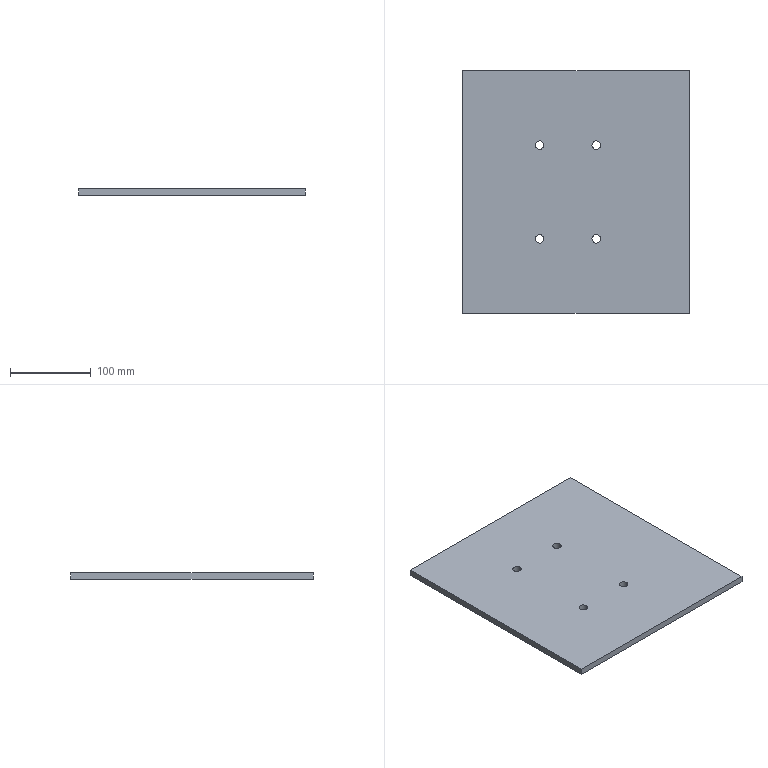Part | SolidWorks | features Extrusion 1, ICE 1 | 1 solid | 14 faces | box 280 x 300 x 8 mm | volume 669229 mm3 | cylinder 8 | plane 6 | commonest cylinder face diameters 10.5 x8
STEP:
#1=CARTESIAN_POINT('',(88.648,-50.185,8.));
#2=VERTEX_POINT('',#1);
#3=CARTESIAN_POINT('',(78.148,-50.185,8.));
#4=VERTEX_POINT('',#3);
#5=CARTESIAN_POINT('',(83.398,-50.185,8.));
#6=DIRECTION('',(0.,0.,-1.));
#7=DIRECTION('',(-1.,0.,0.));
#8=AXIS2_PLACEMENT_3D('',#5,#6,#7);
#9=CIRCLE('',#8,5.25);
#10=EDGE_CURVE('',#2,#4,#9,.T.);
#11=ORIENTED_EDGE('',*,*,#10,.F.);
#12=CARTESIAN_POINT('',(88.648,-50.185,0.));
#13=VERTEX_POINT('',#12);
#14=CARTESIAN_POINT('',(88.648,-50.185,8.));
#15=DIRECTION('',(0.,0.,-1.));
#16=VECTOR('',#15,1000.);
#17=LINE('',#14,#16);
#18=EDGE_CURVE('',#2,#13,#17,.T.);
#19=ORIENTED_EDGE('',*,*,#18,.T.);
#20=CARTESIAN_POINT('',(78.148,-50.185,0.));
#21=VERTEX_POINT('',#20);
#22=CARTESIAN_POINT('',(83.398,-50.185,0.));
#23=DIRECTION('',(0.,0.,-1.));
#24=DIRECTION('',(-1.,0.,0.));
#25=AXIS2_PLACEMENT_3D('',#22,#23,#24);
#26=CIRCLE('',#25,5.25);
#27=EDGE_CURVE('',#13,#21,#26,.T.);
#28=ORIENTED_EDGE('',*,*,#27,.T.);
#29=CARTESIAN_POINT('',(78.148,-50.185,8.));
#30=DIRECTION('',(0.,0.,-1.));
#31=VECTOR('',#30,1000.);
#32=LINE('',#29,#31);
#33=EDGE_CURVE('',#4,#21,#32,.T.);
#34=ORIENTED_EDGE('',*,*,#33,.F.);
#35=EDGE_LOOP('',(#11,#19,#28,#34));
#36=FACE_OUTER_BOUND('',#35,.T.);
#37=CARTESIAN_POINT('',(83.398,-50.185,8.));
#38=DIRECTION('',(0.,0.,-1.));
#39=DIRECTION('',(-1.,0.,0.));
#40=AXIS2_PLACEMENT_3D('',#37,#38,#39);
#41=CYLINDRICAL_SURFACE('',#40,5.25);
#42=ADVANCED_FACE('',(#36),#41,.F.);
#43=CARTESIAN_POINT('',(18.648,-166.185,8.));
#44=VERTEX_POINT('',#43);
#45=CARTESIAN_POINT('',(8.148,-166.185,8.));
#46=VERTEX_POINT('',#45);
#47=CARTESIAN_POINT('',(13.398,-166.185,8.));
#48=DIRECTION('',(0.,0.,-1.));
#49=DIRECTION('',(1.,0.,0.));
#50=AXIS2_PLACEMENT_3D('',#47,#48,#49);
#51=CIRCLE('',#50,5.25);
#52=EDGE_CURVE('',#44,#46,#51,.T.);
#53=ORIENTED_EDGE('',*,*,#52,.F.);
#54=CARTESIAN_POINT('',(18.648,-166.185,0.));
#55=VERTEX_POINT('',#54);
#56=CARTESIAN_POINT('',(18.648,-166.185,8.));
#57=DIRECTION('',(0.,0.,-1.));
#58=VECTOR('',#57,1000.);
#59=LINE('',#56,#58);
#60=EDGE_CURVE('',#44,#55,#59,.T.);
#61=ORIENTED_EDGE('',*,*,#60,.T.);
#62=CARTESIAN_POINT('',(8.148,-166.185,0.));
#63=VERTEX_POINT('',#62);
#64=CARTESIAN_POINT('',(13.398,-166.185,0.));
#65=DIRECTION('',(0.,0.,-1.));
#66=DIRECTION('',(1.,0.,0.));
#67=AXIS2_PLACEMENT_3D('',#64,#65,#66);
#68=CIRCLE('',#67,5.25);
#69=EDGE_CURVE('',#55,#63,#68,.T.);
#70=ORIENTED_EDGE('',*,*,#69,.T.);
#71=CARTESIAN_POINT('',(8.148,-166.185,8.));
#72=DIRECTION('',(0.,0.,-1.));
#73=VECTOR('',#72,1000.);
#74=LINE('',#71,#73);
#75=EDGE_CURVE('',#46,#63,#74,.T.);
#76=ORIENTED_EDGE('',*,*,#75,.F.);
#77=EDGE_LOOP('',(#53,#61,#70,#76));
#78=FACE_OUTER_BOUND('',#77,.T.);
#79=CARTESIAN_POINT('',(13.398,-166.185,8.));
#80=DIRECTION('',(0.,0.,-1.));
#81=DIRECTION('',(-1.,0.,0.));
#82=AXIS2_PLACEMENT_3D('',#79,#80,#81);
#83=CYLINDRICAL_SURFACE('',#82,5.25);
#84=ADVANCED_FACE('',(#78),#83,.F.);
#85=CARTESIAN_POINT('',(88.648,-166.185,8.));
#86=VERTEX_POINT('',#85);
#87=CARTESIAN_POINT('',(78.148,-166.185,8.));
#88=VERTEX_POINT('',#87);
#89=CARTESIAN_POINT('',(83.398,-166.185,8.));
#90=DIRECTION('',(0.,0.,-1.));
#91=DIRECTION('',(1.,0.,0.));
#92=AXIS2_PLACEMENT_3D('',#89,#90,#91);
#93=CIRCLE('',#92,5.25);
#94=EDGE_CURVE('',#86,#88,#93,.T.);
#95=ORIENTED_EDGE('',*,*,#94,.F.);
#96=CARTESIAN_POINT('',(88.648,-166.185,0.));
#97=VERTEX_POINT('',#96);
#98=CARTESIAN_POINT('',(88.648,-166.185,8.));
#99=DIRECTION('',(0.,0.,-1.));
#100=VECTOR('',#99,1000.);
#101=LINE('',#98,#100);
#102=EDGE_CURVE('',#86,#97,#101,.T.);
#103=ORIENTED_EDGE('',*,*,#102,.T.);
#104=CARTESIAN_POINT('',(78.148,-166.185,0.));
#105=VERTEX_POINT('',#104);
#106=CARTESIAN_POINT('',(83.398,-166.185,0.));
#107=DIRECTION('',(0.,0.,-1.));
#108=DIRECTION('',(1.,0.,0.));
#109=AXIS2_PLACEMENT_3D('',#106,#107,#108);
#110=CIRCLE('',#109,5.25);
#111=EDGE_CURVE('',#97,#105,#110,.T.);
#112=ORIENTED_EDGE('',*,*,#111,.T.);
#113=CARTESIAN_POINT('',(78.148,-166.185,8.));
#114=DIRECTION('',(0.,0.,-1.));
#115=VECTOR('',#114,1000.);
#116=LINE('',#113,#115);
#117=EDGE_CURVE('',#88,#105,#116,.T.);
#118=ORIENTED_EDGE('',*,*,#117,.F.);
#119=EDGE_LOOP('',(#95,#103,#112,#118));
#120=FACE_OUTER_BOUND('',#119,.T.);
#121=CARTESIAN_POINT('',(83.398,-166.185,8.));
#122=DIRECTION('',(0.,0.,-1.));
#123=DIRECTION('',(-1.,0.,0.));
#124=AXIS2_PLACEMENT_3D('',#121,#122,#123);
#125=CYLINDRICAL_SURFACE('',#124,5.25);
#126=ADVANCED_FACE('',(#120),#125,.F.);
#127=CARTESIAN_POINT('',(18.648,-50.185,8.));
#128=VERTEX_POINT('',#127);
#129=CARTESIAN_POINT('',(8.148,-50.185,8.));
#130=VERTEX_POINT('',#129);
#131=CARTESIAN_POINT('',(13.398,-50.185,8.));
#132=DIRECTION('',(0.,0.,-1.));
#133=DIRECTION('',(-1.,0.,0.));
#134=AXIS2_PLACEMENT_3D('',#131,#132,#133);
#135=CIRCLE('',#134,5.25);
#136=EDGE_CURVE('',#128,#130,#135,.T.);
#137=ORIENTED_EDGE('',*,*,#136,.F.);
#138=CARTESIAN_POINT('',(18.648,-50.185,0.));
#139=VERTEX_POINT('',#138);
#140=CARTESIAN_POINT('',(18.648,-50.185,8.));
#141=DIRECTION('',(0.,0.,-1.));
#142=VECTOR('',#141,1000.);
#143=LINE('',#140,#142);
#144=EDGE_CURVE('',#128,#139,#143,.T.);
#145=ORIENTED_EDGE('',*,*,#144,.T.);
#146=CARTESIAN_POINT('',(8.148,-50.185,0.));
#147=VERTEX_POINT('',#146);
#148=CARTESIAN_POINT('',(13.398,-50.185,0.));
#149=DIRECTION('',(0.,0.,-1.));
#150=DIRECTION('',(-1.,0.,0.));
#151=AXIS2_PLACEMENT_3D('',#148,#149,#150);
#152=CIRCLE('',#151,5.25);
#153=EDGE_CURVE('',#139,#147,#152,.T.);
#154=ORIENTED_EDGE('',*,*,#153,.T.);
#155=CARTESIAN_POINT('',(8.148,-50.185,8.));
#156=DIRECTION('',(0.,0.,-1.));
#157=VECTOR('',#156,1000.);
#158=LINE('',#155,#157);
#159=EDGE_CURVE('',#130,#147,#158,.T.);
#160=ORIENTED_EDGE('',*,*,#159,.F.);
#161=EDGE_LOOP('',(#137,#145,#154,#160));
#162=FACE_OUTER_BOUND('',#161,.T.);
#163=CARTESIAN_POINT('',(13.398,-50.185,8.));
#164=DIRECTION('',(0.,0.,-1.));
#165=DIRECTION('',(-1.,0.,0.));
#166=AXIS2_PLACEMENT_3D('',#163,#164,#165);
#167=CYLINDRICAL_SURFACE('',#166,5.25);
#168=ADVANCED_FACE('',(#162),#167,.F.);
#169=CARTESIAN_POINT('',(-81.602,41.815,0.));
#170=VERTEX_POINT('',#169);
#171=CARTESIAN_POINT('',(-81.602,-258.185,0.));
#172=VERTEX_POINT('',#171);
#173=CARTESIAN_POINT('',(-81.602,41.815,0.));
#174=DIRECTION('',(0.,-1.,0.));
#175=VECTOR('',#174,1000.);
#176=LINE('',#173,#175);
#177=EDGE_CURVE('',#170,#172,#176,.T.);
#178=ORIENTED_EDGE('',*,*,#177,.T.);
#179=CARTESIAN_POINT('',(-81.602,-258.185,8.));
#180=VERTEX_POINT('',#179);
#181=CARTESIAN_POINT('',(-81.602,-258.185,8.));
#182=DIRECTION('',(0.,0.,-1.));
#183=VECTOR('',#182,1000.);
#184=LINE('',#181,#183);
#185=EDGE_CURVE('',#180,#172,#184,.T.);
#186=ORIENTED_EDGE('',*,*,#185,.F.);
#187=CARTESIAN_POINT('',(-81.602,41.815,8.));
#188=VERTEX_POINT('',#187);
#189=CARTESIAN_POINT('',(-81.602,41.815,8.));
#190=DIRECTION('',(0.,-1.,0.));
#191=VECTOR('',#190,1000.);
#192=LINE('',#189,#191);
#193=EDGE_CURVE('',#188,#180,#192,.T.);
#194=ORIENTED_EDGE('',*,*,#193,.F.);
#195=CARTESIAN_POINT('',(-81.602,41.815,8.));
#196=DIRECTION('',(0.,0.,-1.));
#197=VECTOR('',#196,1000.);
#198=LINE('',#195,#197);
#199=EDGE_CURVE('',#188,#170,#198,.T.);
#200=ORIENTED_EDGE('',*,*,#199,.T.);
#201=EDGE_LOOP('',(#178,#186,#194,#200));
#202=FACE_OUTER_BOUND('',#201,.T.);
#203=CARTESIAN_POINT('',(-81.602,41.815,8.));
#204=DIRECTION('',(1.,0.,0.));
#205=DIRECTION('',(0.,1.,0.));
#206=AXIS2_PLACEMENT_3D('',#203,#204,#205);
#207=PLANE('',#206);
#208=ADVANCED_FACE('',(#202),#207,.F.);
#209=CARTESIAN_POINT('',(198.398,-258.185,0.));
#210=VERTEX_POINT('',#209);
#211=CARTESIAN_POINT('',(-81.602,-258.185,0.));
#212=DIRECTION('',(1.,0.,0.));
#213=VECTOR('',#212,1000.);
#214=LINE('',#211,#213);
#215=EDGE_CURVE('',#172,#210,#214,.T.);
#216=ORIENTED_EDGE('',*,*,#215,.T.);
#217=CARTESIAN_POINT('',(198.398,-258.185,8.));
#218=VERTEX_POINT('',#217);
#219=CARTESIAN_POINT('',(198.398,-258.185,8.));
#220=DIRECTION('',(0.,0.,-1.));
#221=VECTOR('',#220,1000.);
#222=LINE('',#219,#221);
#223=EDGE_CURVE('',#218,#210,#222,.T.);
#224=ORIENTED_EDGE('',*,*,#223,.F.);
#225=CARTESIAN_POINT('',(-81.602,-258.185,8.));
#226=DIRECTION('',(1.,0.,0.));
#227=VECTOR('',#226,1000.);
#228=LINE('',#225,#227);
#229=EDGE_CURVE('',#180,#218,#228,.T.);
#230=ORIENTED_EDGE('',*,*,#229,.F.);
#231=ORIENTED_EDGE('',*,*,#185,.T.);
#232=EDGE_LOOP('',(#216,#224,#230,#231));
#233=FACE_OUTER_BOUND('',#232,.T.);
#234=CARTESIAN_POINT('',(-81.602,-258.185,8.));
#235=DIRECTION('',(0.,1.,0.));
#236=DIRECTION('',(0.,0.,1.));
#237=AXIS2_PLACEMENT_3D('',#234,#235,#236);
#238=PLANE('',#237);
#239=ADVANCED_FACE('',(#233),#238,.F.);
#240=CARTESIAN_POINT('',(198.398,41.815,0.));
#241=VERTEX_POINT('',#240);
#242=CARTESIAN_POINT('',(198.398,41.815,0.));
#243=DIRECTION('',(0.,1.,0.));
#244=VECTOR('',#243,1000.);
#245=LINE('',#242,#244);
#246=EDGE_CURVE('',#210,#241,#245,.T.);
#247=ORIENTED_EDGE('',*,*,#246,.T.);
#248=CARTESIAN_POINT('',(198.398,41.815,8.));
#249=VERTEX_POINT('',#248);
#250=CARTESIAN_POINT('',(198.398,41.815,8.));
#251=DIRECTION('',(0.,0.,-1.));
#252=VECTOR('',#251,1000.);
#253=LINE('',#250,#252);
#254=EDGE_CURVE('',#249,#241,#253,.T.);
#255=ORIENTED_EDGE('',*,*,#254,.F.);
#256=CARTESIAN_POINT('',(198.398,41.815,8.));
#257=DIRECTION('',(0.,1.,0.));
#258=VECTOR('',#257,1000.);
#259=LINE('',#256,#258);
#260=EDGE_CURVE('',#218,#249,#259,.T.);
#261=ORIENTED_EDGE('',*,*,#260,.F.);
#262=ORIENTED_EDGE('',*,*,#223,.T.);
#263=EDGE_LOOP('',(#247,#255,#261,#262));
#264=FACE_OUTER_BOUND('',#263,.T.);
#265=CARTESIAN_POINT('',(198.398,41.815,8.));
#266=DIRECTION('',(-1.,0.,0.));
#267=DIRECTION('',(0.,-1.,0.));
#268=AXIS2_PLACEMENT_3D('',#265,#266,#267);
#269=PLANE('',#268);
#270=ADVANCED_FACE('',(#264),#269,.F.);
#271=CARTESIAN_POINT('',(-81.602,41.815,0.));
#272=DIRECTION('',(-1.,0.,0.));
#273=VECTOR('',#272,1000.);
#274=LINE('',#271,#273);
#275=EDGE_CURVE('',#241,#170,#274,.T.);
#276=ORIENTED_EDGE('',*,*,#275,.T.);
#277=ORIENTED_EDGE('',*,*,#199,.F.);
#278=CARTESIAN_POINT('',(-81.602,41.815,8.));
#279=DIRECTION('',(-1.,0.,0.));
#280=VECTOR('',#279,1000.);
#281=LINE('',#278,#280);
#282=EDGE_CURVE('',#249,#188,#281,.T.);
#283=ORIENTED_EDGE('',*,*,#282,.F.);
#284=ORIENTED_EDGE('',*,*,#254,.T.);
#285=EDGE_LOOP('',(#276,#277,#283,#284));
#286=FACE_OUTER_BOUND('',#285,.T.);
#287=CARTESIAN_POINT('',(-81.602,41.815,8.));
#288=DIRECTION('',(0.,-1.,0.));
#289=DIRECTION('',(0.,0.,-1.));
#290=AXIS2_PLACEMENT_3D('',#287,#288,#289);
#291=PLANE('',#290);
#292=ADVANCED_FACE('',(#286),#291,.F.);
#293=CARTESIAN_POINT('',(83.398,-50.185,8.));
#294=DIRECTION('',(0.,0.,-1.));
#295=DIRECTION('',(-1.,0.,0.));
#296=AXIS2_PLACEMENT_3D('',#293,#294,#295);
#297=CIRCLE('',#296,5.25);
#298=EDGE_CURVE('',#4,#2,#297,.T.);
#299=ORIENTED_EDGE('',*,*,#298,.T.);
#300=ORIENTED_EDGE('',*,*,#10,.T.);
#301=EDGE_LOOP('',(#299,#300));
#302=FACE_BOUND('',#301,.T.);
#303=CARTESIAN_POINT('',(13.398,-166.185,8.));
#304=DIRECTION('',(0.,0.,-1.));
#305=DIRECTION('',(1.,0.,0.));
#306=AXIS2_PLACEMENT_3D('',#303,#304,#305);
#307=CIRCLE('',#306,5.25);
#308=EDGE_CURVE('',#46,#44,#307,.T.);
#309=ORIENTED_EDGE('',*,*,#308,.T.);
#310=ORIENTED_EDGE('',*,*,#52,.T.);
#311=EDGE_LOOP('',(#309,#310));
#312=FACE_BOUND('',#311,.T.);
#313=CARTESIAN_POINT('',(83.398,-166.185,8.));
#314=DIRECTION('',(0.,0.,-1.));
#315=DIRECTION('',(1.,0.,0.));
#316=AXIS2_PLACEMENT_3D('',#313,#314,#315);
#317=CIRCLE('',#316,5.25);
#318=EDGE_CURVE('',#88,#86,#317,.T.);
#319=ORIENTED_EDGE('',*,*,#318,.T.);
#320=ORIENTED_EDGE('',*,*,#94,.T.);
#321=EDGE_LOOP('',(#319,#320));
#322=FACE_BOUND('',#321,.T.);
#323=CARTESIAN_POINT('',(13.398,-50.185,8.));
#324=DIRECTION('',(0.,0.,-1.));
#325=DIRECTION('',(-1.,0.,0.));
#326=AXIS2_PLACEMENT_3D('',#323,#324,#325);
#327=CIRCLE('',#326,5.25);
#328=EDGE_CURVE('',#130,#128,#327,.T.);
#329=ORIENTED_EDGE('',*,*,#328,.T.);
#330=ORIENTED_EDGE('',*,*,#136,.T.);
#331=EDGE_LOOP('',(#329,#330));
#332=FACE_BOUND('',#331,.T.);
#333=ORIENTED_EDGE('',*,*,#193,.T.);
#334=ORIENTED_EDGE('',*,*,#229,.T.);
#335=ORIENTED_EDGE('',*,*,#260,.T.);
#336=ORIENTED_EDGE('',*,*,#282,.T.);
#337=EDGE_LOOP('',(#333,#334,#335,#336));
#338=FACE_OUTER_BOUND('',#337,.T.);
#339=CARTESIAN_POINT('',(0.,0.,8.));
#340=DIRECTION('',(0.,0.,1.));
#341=DIRECTION('',(1.,0.,0.));
#342=AXIS2_PLACEMENT_3D('',#339,#340,#341);
#343=PLANE('',#342);
#344=ADVANCED_FACE('',(#302,#312,#322,#332,#338),#343,.T.);
#345=CARTESIAN_POINT('',(83.398,-50.185,0.));
#346=DIRECTION('',(0.,0.,-1.));
#347=DIRECTION('',(-1.,0.,0.));
#348=AXIS2_PLACEMENT_3D('',#345,#346,#347);
#349=CIRCLE('',#348,5.25);
#350=EDGE_CURVE('',#21,#13,#349,.T.);
#351=ORIENTED_EDGE('',*,*,#350,.F.);
#352=ORIENTED_EDGE('',*,*,#27,.F.);
#353=EDGE_LOOP('',(#351,#352));
#354=FACE_BOUND('',#353,.T.);
#355=CARTESIAN_POINT('',(13.398,-166.185,0.));
#356=DIRECTION('',(0.,0.,-1.));
#357=DIRECTION('',(1.,0.,0.));
#358=AXIS2_PLACEMENT_3D('',#355,#356,#357);
#359=CIRCLE('',#358,5.25);
#360=EDGE_CURVE('',#63,#55,#359,.T.);
#361=ORIENTED_EDGE('',*,*,#360,.F.);
#362=ORIENTED_EDGE('',*,*,#69,.F.);
#363=EDGE_LOOP('',(#361,#362));
#364=FACE_BOUND('',#363,.T.);
#365=CARTESIAN_POINT('',(83.398,-166.185,0.));
#366=DIRECTION('',(0.,0.,-1.));
#367=DIRECTION('',(1.,0.,0.));
#368=AXIS2_PLACEMENT_3D('',#365,#366,#367);
#369=CIRCLE('',#368,5.25);
#370=EDGE_CURVE('',#105,#97,#369,.T.);
#371=ORIENTED_EDGE('',*,*,#370,.F.);
#372=ORIENTED_EDGE('',*,*,#111,.F.);
#373=EDGE_LOOP('',(#371,#372));
#374=FACE_BOUND('',#373,.T.);
#375=CARTESIAN_POINT('',(13.398,-50.185,0.));
#376=DIRECTION('',(0.,0.,-1.));
#377=DIRECTION('',(-1.,0.,0.));
#378=AXIS2_PLACEMENT_3D('',#375,#376,#377);
#379=CIRCLE('',#378,5.25);
#380=EDGE_CURVE('',#147,#139,#379,.T.);
#381=ORIENTED_EDGE('',*,*,#380,.F.);
#382=ORIENTED_EDGE('',*,*,#153,.F.);
#383=EDGE_LOOP('',(#381,#382));
#384=FACE_BOUND('',#383,.T.);
#385=ORIENTED_EDGE('',*,*,#177,.F.);
#386=ORIENTED_EDGE('',*,*,#275,.F.);
#387=ORIENTED_EDGE('',*,*,#246,.F.);
#388=ORIENTED_EDGE('',*,*,#215,.F.);
#389=EDGE_LOOP('',(#385,#386,#387,#388));
#390=FACE_OUTER_BOUND('',#389,.T.);
#391=CARTESIAN_POINT('',(0.,0.,0.));
#392=DIRECTION('',(0.,0.,1.));
#393=DIRECTION('',(1.,0.,0.));
#394=AXIS2_PLACEMENT_3D('',#391,#392,#393);
#395=PLANE('',#394);
#396=ADVANCED_FACE('',(#354,#364,#374,#384,#390),#395,.F.);
#397=ORIENTED_EDGE('',*,*,#144,.F.);
#398=ORIENTED_EDGE('',*,*,#328,.F.);
#399=ORIENTED_EDGE('',*,*,#159,.T.);
#400=ORIENTED_EDGE('',*,*,#380,.T.);
#401=EDGE_LOOP('',(#397,#398,#399,#400));
#402=FACE_OUTER_BOUND('',#401,.T.);
#403=CARTESIAN_POINT('',(13.398,-50.185,8.));
#404=DIRECTION('',(0.,0.,-1.));
#405=DIRECTION('',(-1.,0.,0.));
#406=AXIS2_PLACEMENT_3D('',#403,#404,#405);
#407=CYLINDRICAL_SURFACE('',#406,5.25);
#408=ADVANCED_FACE('',(#402),#407,.F.);
#409=ORIENTED_EDGE('',*,*,#102,.F.);
#410=ORIENTED_EDGE('',*,*,#318,.F.);
#411=ORIENTED_EDGE('',*,*,#117,.T.);
#412=ORIENTED_EDGE('',*,*,#370,.T.);
#413=EDGE_LOOP('',(#409,#410,#411,#412));
#414=FACE_OUTER_BOUND('',#413,.T.);
#415=CARTESIAN_POINT('',(83.398,-166.185,8.));
#416=DIRECTION('',(0.,0.,-1.));
#417=DIRECTION('',(-1.,0.,0.));
#418=AXIS2_PLACEMENT_3D('',#415,#416,#417);
#419=CYLINDRICAL_SURFACE('',#418,5.25);
#420=ADVANCED_FACE('',(#414),#419,.F.);
#421=ORIENTED_EDGE('',*,*,#60,.F.);
#422=ORIENTED_EDGE('',*,*,#308,.F.);
#423=ORIENTED_EDGE('',*,*,#75,.T.);
#424=ORIENTED_EDGE('',*,*,#360,.T.);
#425=EDGE_LOOP('',(#421,#422,#423,#424));
#426=FACE_OUTER_BOUND('',#425,.T.);
#427=CARTESIAN_POINT('',(13.398,-166.185,8.));
#428=DIRECTION('',(0.,0.,-1.));
#429=DIRECTION('',(-1.,0.,0.));
#430=AXIS2_PLACEMENT_3D('',#427,#428,#429);
#431=CYLINDRICAL_SURFACE('',#430,5.25);
#432=ADVANCED_FACE('',(#426),#431,.F.);
#433=ORIENTED_EDGE('',*,*,#18,.F.);
#434=ORIENTED_EDGE('',*,*,#298,.F.);
#435=ORIENTED_EDGE('',*,*,#33,.T.);
#436=ORIENTED_EDGE('',*,*,#350,.T.);
#437=EDGE_LOOP('',(#433,#434,#435,#436));
#438=FACE_OUTER_BOUND('',#437,.T.);
#439=CARTESIAN_POINT('',(83.398,-50.185,8.));
#440=DIRECTION('',(0.,0.,-1.));
#441=DIRECTION('',(-1.,0.,0.));
#442=AXIS2_PLACEMENT_3D('',#439,#440,#441);
#443=CYLINDRICAL_SURFACE('',#442,5.25);
#444=ADVANCED_FACE('',(#438),#443,.F.);
#445=CLOSED_SHELL('',(#42,#84,#126,#168,#208,#239,#270,#292,#344,#396,#408,#420,#432,#444));
#446=MANIFOLD_SOLID_BREP('',#445);
#447=CARTESIAN_POINT('',(0.,0.,0.));
#448=DIRECTION('',(0.,0.,1.));
#449=DIRECTION('',(1.,0.,0.));
#450=AXIS2_PLACEMENT_3D('',#447,#448,#449);
#451=(LENGTH_UNIT()NAMED_UNIT(*)SI_UNIT(.MILLI.,.METRE.));
#452=UNCERTAINTY_MEASURE_WITH_UNIT(LENGTH_MEASURE(0.00001),#451,'','');
#453=(NAMED_UNIT(*)PLANE_ANGLE_UNIT()SI_UNIT($,.RADIAN.));
#454=(NAMED_UNIT(*)SI_UNIT($,.STERADIAN.)SOLID_ANGLE_UNIT());
#455=(GEOMETRIC_REPRESENTATION_CONTEXT(3)GLOBAL_UNCERTAINTY_ASSIGNED_CONTEXT((#452))GLOBAL_UNIT_ASSIGNED_CONTEXT((#451,#453,#454))REPRESENTATION_CONTEXT('',''));
#456=ADVANCED_BREP_SHAPE_REPRESENTATION('',(#446,#450),#455);